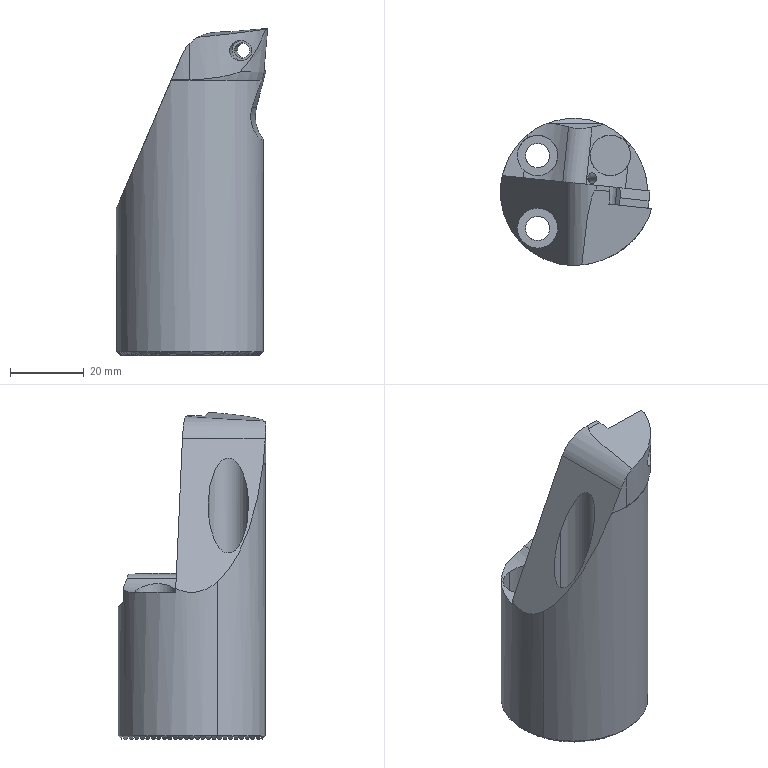NC program | Mastercam | posted with a generic post
Lines 22 to 750 of 11394:
(12 FEMR |TOOL - 1|DIA. OFF. - 1|LEN. - 1|TOOL DIA. - 12.)
N108 T1 M6
N110 G0 G55 G90 X47.529 Y29.275 C6. B-90. S3500 M3
N112 G43 H1 Z102.44
N114 Z4.44
N116 G1 Z2.69 F2000.
N118 X46.832 Y27.706 Z2.539 F2800.
N120 G3 X46.6 Y26.61 Z2.44 I2.468 J-1.096
N122 G1 Y26.
N124 X46.857 Y25.933
N126 G3 X49.366 Y25.751 I2.719 J20.13
N128 X56.385 Y25.697 I7.019 J457.418
N130 X58.173 Y25.7 J457.472
N132 G1 X58.58
N134 X73.217 Y25.712
N136 G3 X74.788 Y25.96 I-1.559 J14.923
N138 G2 X79.594 Y26.531 I10.889 J-71.178
N140 X85.304 Y27.044 I90.742 J-978.65
N142 G1 X85.71 Y27.079
N144 G2 X88.612 Y27.319 I14.877 J-162.688
N146 G1 X88.648
N148 G2 X91.848 Y26.431 J-6.209
N150 X94.413 Y23.878 I-3.935 J-6.52
N152 X95.771 Y20.319 I-9.343 J-5.604
N154 X96.172 Y16.703 I-22.913 J-4.367
N156 X96.263 Y11.23 I-164.754 J-5.473
N158 X96.26 Y10.372 I-164.845
N160 G1 X96.261 Y9.963
N162 X96.262 Y-20.063
N164 G2 X95.238 Y-23.24 I-6.113 J.217
N166 X92.516 Y-25.695 I-6.144 J4.075
N168 X89.126 Y-26.78 I-4.792 J9.131
N170 X86.426 Y-26.964 I-2.7 J19.725
N172 X85.595 Y-26.947 J19.909
N174 X80.026 Y-26.576 I4.415 J108.3
N176 X77.254 Y-26.296 I3.443 J47.898
N178 X75.239 Y-25.92 I6.779 J41.994
N180 G3 X72.669 Y-25.747 I-2.789 J-22.233
N182 X65.45 Y-25.696 I-7.219 J-514.472
N184 X63.445 Y-25.7 J-514.523
N186 G1 X63.038
N188 X46.6
N190 Y-26.514
N192 G3 X46.832 Y-27.609 Z2.514 I2.7
N194 G1 X47.529 Y-29.179 Z2.628
N196 G3 X47.993 Y-29.977 Z2.69 I3.871 J1.719
N198 X51.4 Y-31.696 I3.407 J2.517
N200 X51.486 Y-31.695 J4.236
N202 G1 X85.77 Y-31. F9500.
N204 G3 X97.868 Y-18.729 I-.251 J12.346
N206 G1 X98.099 Y19.214
N208 Y19.274
N210 G3 X88.634 Y29.049 I-9.78
N212 G1 X49.187 Y30.319
N214 G3 X49.132 Y30.32 I-.055 J-1.727
N216 X48.085 Y29.967 J-1.728
N218 X47.552 Y29.293 Z2.632 I1.047 J-1.375 F2800.
N220 G1 X47.529 Y29.241 Z2.628
N222 X46.832 Y27.672 Z2.514
N224 G3 X46.6 Y26.576 Z2.44 I2.468 J-1.096
N226 G1 Y25.966
N228 Y25.941
N230 G3 X47.322 Y25.742 I1.184 J2.896
N232 X50.202 Y25.481 I3.284 J20.205
N234 X56.326 Y25.4 I6.124 J231.975
N236 X57.331 Y25.403 J232.056
N238 G1 X57.737 Y25.402
N240 X71.868 Y25.405
N242 G3 X74.16 Y25.606 I-.455 J18.407
N244 G1 X74.56 Y25.656
N246 G2 X83.654 Y26.595 I27.944 J-226.233
N248 G1 X84.061 Y26.631
N250 G2 X86.741 Y26.858 I16.424 J-178.336
N252 X87.052 Y26.864 I.311 J-7.716
N254 X92.353 Y24.757 J-7.722
N256 X94.693 Y21.289 I-6.626 J-6.994
N258 X95.57 Y17.974 I-13.452 J-5.331
N260 X95.9 Y13.699 I-34.856 J-4.848
N262 X95.966 Y6.255 I-422.145 J-7.444
N264 X95.963 Y4.599 I-422.211
N266 G1 Y4.192
N268 X95.951 Y-18.459
N270 G2 X93.339 Y-23.853 I-7.737 J.417
N272 X89.684 Y-25.862 I-6.391 J7.299
N274 X86.31 Y-26.439 I-4.126 J13.967
N276 X84.545 Y-26.483 I-1.765 J35.346
N278 X82.028 Y-26.394 J35.39
N280 X77.974 Y-26.036 I2.926 J56.249
N282 G3 X74.974 Y-25.628 I-8.378 J-50.369
N284 X70.119 Y-25.427 I-4.903 J-59.734
N286 X62.633 Y-25.399 I-7.486 J-999.104
N288 X60.821 Y-25.4 J-999.132
N290 G1 X60.415
N292 X47.626 Y-25.411
N294 G3 X46.6 Y-25.508 I1.118 J-17.319
N296 G1 Y-25.915
N298 Y-26.322
N300 G3 X46.832 Y-27.418 Z2.514 I2.7
N302 G1 X47.529 Y-28.987 Z2.628
N304 G3 X47.967 Y-29.801 Z2.69 I5.542 J2.46
N306 X53.071 Y-32.591 I5.104 J3.274 F9500.
N308 X53.716 Y-32.556 J6.064
N310 G1 X86.509 Y-29.048
N312 G3 X97.568 Y-16.768 I-1.317 J12.305
N314 G1 X97.634 Y17.323
N316 Y17.345
N318 G3 X87.026 Y28.482 I-11.15
N320 G1 X49.293 Y30.322
N322 G3 X49.206 Y30.324 I-.087 J-1.793
N324 X48.066 Y29.915 J-1.795
N326 X47.566 Y29.257 Z2.634 I1.14 J-1.386 F2800.
N328 G1 X47.529 Y29.175 Z2.628
N330 X46.832 Y27.605 Z2.514
N332 G3 X46.6 Y26.51 Z2.44 I2.468 J-1.095
N334 G1 Y25.899
N336 Y25.867
N338 G3 X47.295 Y25.621 I1.309 J2.597
N340 X49.974 Y25.257 I3.398 J14.942
N342 X55.219 Y25.116 I5.245 J97.179
N344 X55.353 Y25.115 J97.32
N346 X60.423 Y25.101 I5.07 J930.161
N348 G1 X60.613
N350 X61.019
N352 X71.071 Y25.112
N354 G3 X74.684 Y25.394 I-1.302 J39.973
N356 X75.486 Y25.482 I-69.31 J635.193
N358 G2 X85.35 Y26.427 I36.383 J-327.653
N360 X85.873 Y26.443 I.523 J-8.656
N362 X92.552 Y23.301 J-8.672
N364 X94.646 Y19.395 I-8.696 J-7.175
N366 X95.414 Y15.35 I-18.846 J-5.675
N368 X95.636 Y10.046 I-67.384 J-5.48
N370 X95.664 Y2.602 I-985.697 J-7.444
N372 X95.663 Y1.031 I-985.725
N374 G1 Y.624
N376 X95.654 Y-16.85
N378 G2 X94.481 Y-21.108 I-8.896 J.161
N380 X91.007 Y-24.46 I-7.788 J4.595
N382 X87.055 Y-25.793 I-5.819 J10.73
N384 X83.54 Y-26.06 I-3.515 J23.029
N386 X82.887 Y-26.05 J23.296
N388 X77.474 Y-25.624 I.753 J44.179
N390 G3 X70.31 Y-25.146 I-7.489 J-58.236
N392 X60.515 Y-25.097 I-9.795 J-973.891
N394 X57.787 Y-25.1 J-973.94
N396 G1 X57.38
N398 X48.93 Y-25.107
N400 G3 X47.249 Y-25.217 I.087 J-14.256
N402 G2 X46.6 Y-25.332 I-4.342 J22.51
N404 G1 Y-25.739
N406 Y-26.146
N408 G3 X46.832 Y-27.242 Z2.514 I2.7
N410 G1 X47.529 Y-28.811 Z2.628
N412 G3 X47.967 Y-29.625 Z2.69 I5.563 J2.47
N414 X53.092 Y-32.428 I5.125 J3.284 F9500.
N416 X54.034 Y-32.355 J6.087
N418 G1 X86.769 Y-27.226
N420 G3 X97.268 Y-15.041 I-1.923 J12.272
N422 G1 X97.485 Y15.883
N424 Y15.968
N426 G3 X86.059 Y28.113 I-12.167
N428 G1 X49.574 Y30.338
N430 G3 X49.446 Y30.342 I-.128 J-2.094
N432 X48.075 Y29.832 J-2.098
N434 X47.529 Y29.095 Z2.628 I1.371 J-1.588 F2800.
N436 G1 X46.832 Y27.526 Z2.514
N438 G3 X46.6 Y26.43 Z2.44 I2.468 J-1.096
N440 G1 Y25.82
N442 Y25.783
N444 G3 X47.27 Y25.501 I1.407 J2.405
N446 X49.799 Y25.047 I3.498 J12.216
N448 X54.651 Y24.836 I5.066 J60.597
N450 X63.195 Y24.799 I8.544 J976.208
N452 X65.158 Y24.8 J976.245
N454 G1 X65.565
N456 G3 X66.808 Y24.797 I1.243 J274.393
N458 X70.699 Y24.825 J274.396
N460 X75.601 Y25.204 I-2.579 J65.269
N462 G1 X76.004 Y25.245
N464 G2 X83.915 Y26. I42.144 J-400.038
N466 X84.724 Y26.031 I.809 J-10.529
N468 X87.755 Y25.586 J-10.56
N470 X92.529 Y22.101 I-2.915 J-9.004
N472 X94.427 Y18.073 I-10.224 J-7.28
N474 X95.128 Y13.927 I-21.982 J-5.849
N476 X95.339 Y8.254 I-78.186 J-5.743
N478 X95.364 Y1.244 I-984.987 J-7.01
N480 X95.363 Y.062 I-985.012
N482 G1 Y-.345
N484 X95.352 Y-15.565
N486 G2 X94.587 Y-19.353 I-10.488 J.146
N488 X90.687 Y-23.783 I-8.729 J3.753
N490 X86.513 Y-25.312 I-6.351 J10.875
N492 X82.616 Y-25.647 I-3.897 J22.504
N494 X81.802 Y-25.633 J22.839
N496 X77.357 Y-25.289 I2.204 J57.489
N498 G3 X68.875 Y-24.837 I-8.75 J-84.258
N500 X60.513 Y-24.799 I-8.362 J-930.633
N502 X58.769 Y-24.801 J-930.671
N504 G1 X58.362
N506 X49.898 Y-24.808
N508 X49.838
N510 G3 X47.426 Y-24.976 J-17.429
N512 X46.6 Y-25.163 I1.255 J-7.445
N514 G1 Y-25.57
N516 Y-25.977
N518 G3 X46.832 Y-27.073 Z2.514 I2.7
N520 G1 X47.529 Y-28.642 Z2.628
N522 G3 X47.967 Y-29.456 Z2.69 I5.556 J2.466
N524 X53.085 Y-32.255 I5.118 J3.28 F9500.
N526 X54.152 Y-32.161 J6.079
N528 G1 X86.738 Y-26.352
N530 G3 X96.968 Y-14.185 I-2.177 J12.214
N532 G1 X97.079 Y15.053
N534 Y15.101
N536 G3 X85.297 Y27.742 I-12.672
N538 G1 X49.462 Y30.265
N540 G3 X49.328 Y30.27 I-.134 J-1.901
N542 X48.041 Y29.769 J-1.906
N544 X47.586 Y29.137 Z2.638 I1.287 J-1.405 F2800.
N546 G1 X47.529 Y29.008 Z2.628
N548 X46.832 Y27.439 Z2.514
N550 G3 X46.6 Y26.343 Z2.44 I2.468 J-1.096
N552 G1 Y25.733
N554 Y25.692
N556 G3 X47.246 Y25.381 I1.486 J2.256
N558 X49.656 Y24.848 I3.594 J10.545
N560 X53.998 Y24.57 I5.035 J44.572
N562 X62.635 Y24.498 I8.637 J517.551
N564 X64.445 Y24.501 J517.623
N566 G1 X64.852
N568 G3 X66.254 Y24.496 I1.402 J207.057
N570 X70.379 Y24.537 J207.062
N572 X76.13 Y24.965 I-3.438 J85.072
N574 X76.935 Y25.044 I-88.258 J904.631
N576 G1 X77.34 Y25.084
N578 G2 X82.786 Y25.591 I34.321 J-339.181
N580 X83.761 Y25.629 I.975 J-12.402
N582 X86.229 Y25.382 J-12.44
N584 X91.998 Y21.636 I-2.123 J-9.585
N586 X93.961 Y17.697 I-10.303 J-7.593
N588 X94.761 Y13.523 I-20.947 J-6.177
N590 X95.021 Y8.208 I-64.782 J-5.834
N592 X95.067 Y-1.223 I-975.08 J-9.431
N594 X95.063 Y-3.68 I-975.126
N596 G1 Y-4.087
N598 X95.049 Y-14.413
N600 G2 X94.522 Y-17.822 I-12.377 J.17
N602 X90.27 Y-23.216 I-9.382 J3.023
N604 X86.176 Y-24.816 I-6.647 J10.966
N606 X82.02 Y-25.229 I-4.156 J20.707
N608 X81.378 Y-25.22 J21.12
N610 X76.991 Y-24.938 I2.34 J70.796
N612 G3 X67.609 Y-24.531 I-9.629 J-113.557
N614 X60.091 Y-24.501 I-7.518 J-940.281
N616 G1 X59.115
N618 X58.709
N620 G3 X56.458 Y-24.498 I-2.251 J-986.24
N622 X50.281 Y-24.518 J-986.243
N624 X47.503 Y-24.755 I.088 J-17.442
N626 X46.6 Y-24.999 I1.506 J-7.359
N628 G1 Y-25.406
N630 Y-25.813
N632 G3 X46.832 Y-26.909 Z2.514 I2.7
N634 G1 X47.529 Y-28.478 Z2.628
N636 G3 X47.968 Y-29.291 Z2.69 I5.494 J2.439
N638 X53.023 Y-32.05 I5.055 J3.252 F9500.
N640 X53.949 Y-31.978 J6.011
N642 G1 X86.277 Y-26.939
N644 G3 X96.654 Y-14.952 I-1.889 J12.121
N646 G1 X96.965 Y13.493
N648 G3 X96.966 Y13.644 I-13.78 J.151
N650 X84.307 Y27.379 I-13.781
N652 G1 X49.534 Y30.219
N654 G3 X49.376 Y30.225 I-.158 J-1.939
N656 X48.029 Y29.685 J-1.945
N658 X47.597 Y29.069 Z2.639 I1.347 J-1.405 F2800.
N660 G1 X47.529 Y28.916 Z2.628
N662 X46.832 Y27.346 Z2.514
N664 G3 X46.6 Y26.251 Z2.44 I2.468 J-1.095
N666 G1 Y25.64
N668 Y25.597
N670 G3 X47.223 Y25.261 I1.504 J2.039
N672 X49.535 Y24.658 I3.688 J9.408
N674 X53.768 Y24.306 I5.138 J36.114
N676 X61.495 Y24.203 I7.727 J289.202
N678 X62.537 Y24.204 J289.305
N680 G1 X62.942
N682 G3 X64.779 Y24.199 I1.837 J320.857
N684 X69.712 Y24.236 J320.862
N686 X76.27 Y24.686 I-3.143 J93.901
N688 X78.285 Y24.878 I-90.027 J956.941
N690 G1 X78.691 Y24.916
N692 G2 X82.181 Y25.215 I10.21 J-98.931
N694 X82.967 Y25.239 I.786 J-12.621
N696 X85.914 Y24.891 J-12.645
N698 X91.707 Y20.905 I-2.563 J-9.928
N700 X93.505 Y17.335 I-10.653 J-7.603
N702 X94.392 Y13.145 I-20.202 J-6.468
N704 X94.706 Y7.779 I-57.675 J-6.064
N706 X94.767 Y-1.755 I-745.007 J-9.534
N708 X94.763 Y-4.132 I-745.068
N710 G1 Y-4.539
N712 X94.751 Y-13.204
N714 G2 X94.415 Y-16.251 I-14.842 J.094
N716 X89.662 Y-22.806 I-9.994 J2.246
N718 X85.632 Y-24.38 I-6.749 J11.333
N720 X81.446 Y-24.81 I-4.186 J20.176
N722 X81.331 Y-24.809 J20.606
N724 X76.899 Y-24.613 I.618 J63.945
N726 G3 X65.922 Y-24.222 I-10.977 J-153.939
N728 G1 X65.828
N730 G3 X60.162 Y-24.203 I-6.074 J-976.985
N732 G1 X59.756
N734 G3 X57.131 Y-24.199 I-2.625 J-837.057
N736 X50.926 Y-24.222 J-837.061
N738 X48.057 Y-24.442 I.176 J-21.093
N740 X46.6 Y-24.837 I.987 J-6.516
N742 G1 Y-25.244
N744 Y-25.651
N746 G3 X46.832 Y-26.747 Z2.514 I2.7
N748 G1 X47.529 Y-28.316 Z2.628
N750 G3 X47.968 Y-29.129 Z2.69 I5.461 J2.424
N752 X52.99 Y-31.867 I5.022 J3.237 F9500.
N754 X53.937 Y-31.792 J5.975
N756 G1 X86.05 Y-26.64
N758 G3 X96.31 Y-14.865 I-1.931 J12.04
N760 G1 X96.892 Y11.859
N762 G3 X96.895 Y12.18 I-14.731 J.321
N764 X83.594 Y26.844 I-14.734
N766 G1 X49.602 Y30.167
N768 G3 X49.41 Y30.176 I-.192 J-1.958
N770 X48.017 Y29.597 J-1.967
N772 X47.612 Y29.007 Z2.642 I1.393 J-1.388 F2800.
N774 G1 X47.529 Y28.819 Z2.628
N776 X46.832 Y27.25 Z2.514
N778 G3 X46.6 Y26.154 Z2.44 I2.468 J-1.096
N780 G1 Y25.544
N782 Y25.499
N784 G3 X47.202 Y25.14 I1.558 J1.932
N786 X49.431 Y24.474 I3.779 J8.58
N788 X53.564 Y24.048 I5.24 J30.585
N790 X60.61 Y23.911 I7.046 J180.595
N792 G1 X61.061
N794 G3 X63.085 Y23.905 I3.774 J972.824
N796 G1 X63.491
N798 G3 X65.052 Y23.898 I1.561 J184.658
N800 X70.204 Y23.97 J184.665
N802 X77.226 Y24.481 I-5.685 J126.675
N804 X78.032 Y24.556 I-83.251 J898.938
N806 G1 X78.437 Y24.594
N808 G2 X81.574 Y24.838 I6.786 J-66.905
N810 X82.215 Y24.853 I.641 J-13.291
N812 X85.185 Y24.517 J-13.306
N814 X91.413 Y20.216 I-2.521 J-10.31
N816 X93.241 Y16.434 I-11.335 J-7.813
N818 X94.135 Y11.832 I-22.073 J-6.673
N820 X94.416 Y6.113 I-68.472 J-6.238
N822 X94.466 Y-3.799 I-988.079 J-9.912
N824 X94.463 Y-6.183 I-988.129
N826 G1 Y-6.591
N828 G2 X94.466 Y-8.052 I-424.572 J-1.461
N830 X94.443 Y-12.442 I-424.575
N832 X94.043 Y-15.737 I-15.177 J.172
N834 X89.131 Y-22.378 I-10.309 J2.487
N836 X84.862 Y-24.004 I-6.872 J11.631
N838 X80.688 Y-24.405 I-4.174 J21.504
N840 G1 X80.641
N842 G2 X75.848 Y-24.232 I.425 J78.093
N844 G3 X64.583 Y-23.917 I-11.265 J-201.327
N846 G1 X64.307
N848 G3 X60.663 Y-23.905 I-5.051 J-995.672
N850 G1 X60.257 Y-23.904
N852 G3 X57.518 Y-23.898 I-2.739 J-654.676
N854 X51.439 Y-23.927 J-654.682
N856 X48.205 Y-24.195 I.142 J-21.353
N858 X46.6 Y-24.677 I1.11 J-6.602
N860 G1 Y-25.084
N862 Y-25.491
N864 G3 X46.832 Y-26.587 Z2.514 I2.7
N866 G1 X47.529 Y-28.156 Z2.628
N868 G3 X47.968 Y-28.969 Z2.69 I5.497 J2.44
N870 X53.026 Y-31.73 I5.058 J3.253 F9500.
N872 X54.264 Y-31.601 J6.014
N874 G1 X86.304 Y-24.856
N876 G3 X96.048 Y-12.988 I-2.529 J12.01
N878 G1 X96.331 Y11.67
N880 G3 X96.332 Y11.841 I-14.88 J.171
N882 X82.991 Y26.643 I-14.881
N884 G1 X49.669 Y30.111
N886 G3 X49.461 Y30.122 I-.208 J-2.003
N888 X48.009 Y29.503 J-2.014
N890 X47.62 Y28.925 Z2.643 I1.452 J-1.395 F2800.
N892 G1 X47.529 Y28.719 Z2.628
N894 X46.832 Y27.15 Z2.514
N896 G3 X46.6 Y26.054 Z2.44 I2.468 J-1.096
N898 G1 Y25.444
N900 Y25.397
N902 G3 X47.182 Y25.019 I1.601 J1.83
N904 X49.339 Y24.294 I3.864 J7.931
N906 X53.012 Y23.821 I5.101 J25.076
N908 X59.612 Y23.626 I6.695 J114.795
N910 X63.521 Y23.606 I3.909 J377.91
N912 X68.801 Y23.642 J377.93
N914 X76.991 Y24.164 I-3.418 J118.146
N916 G1 X77.393 Y24.2
N918 G2 X80.964 Y24.463 I6.548 J-64.625
N920 X81.518 Y24.474 I.554 J-13.576
N922 X84.842 Y24.062 J-13.587
N924 X90.937 Y19.818 I-2.819 J-10.548
N926 X92.986 Y15.537 I-11.573 J-8.172
N928 X93.83 Y10.997 I-23.493 J-6.715
N930 X94.112 Y5.291 I-70.353 J-6.336
N932 X94.166 Y-4.875 I-951.681 J-10.166
N934 X94.163 Y-7.416 I-951.735
N936 G1 Y-7.824
N938 G2 X94.167 Y-8.784 I-111.645 J-.96
N940 X94.116 Y-12.154 I-111.649
N942 X93.496 Y-15.858 I-14.33 J.496
N944 X88.343 Y-22.12 I-10.435 J3.336
N946 X83.863 Y-23.678 I-6.827 J12.417
N948 X79.729 Y-24.021 I-4.134 J24.752
N950 X79.296 Y-24.017 J25.095
N952 X74.214 Y-23.843 I2.351 J143.346
N954 G3 X62.806 Y-23.61 I-11.408 J-279.326
N956 X62.213 Y-23.611 J-279.559
N958 G1 X61.808 Y-23.61
N960 G3 X58.24 Y-23.601 I-3.568 J-722.458
N962 X52.171 Y-23.626 J-722.467
N964 X48.805 Y-23.868 I.187 J-26.164
N966 X47.012 Y-24.333 I1.095 J-7.901
N968 G1 X46.6 Y-24.519
N970 Y-25.333
N972 G3 X46.832 Y-26.428 Z2.514 I2.7
N974 G1 X47.529 Y-27.998 Z2.628
N976 G3 X47.968 Y-28.811 Z2.69 I5.47 J2.429
N978 X52.999 Y-31.554 I5.031 J3.242 F9500.
N980 X54.274 Y-31.417 J5.985
N982 G1 X86.11 Y-24.477
N984 G3 X95.722 Y-12.734 I-2.601 J11.935
N986 G1 X96.091 Y10.798
N988 G3 X96.093 Y11.035 I-15.119 J.237
N990 X82.79 Y26.046 I-15.121
N992 G1 X49.732 Y30.049
N994 G3 X49.488 Y30.064 I-.244 J-2.011
N996 X47.997 Y29.408 J-2.026
N998 X47.637 Y28.86 Z2.646 I1.491 J-1.37 F2800.
N1000 G1 X47.529 Y28.617 Z2.628
N1002 X46.832 Y27.047 Z2.514
N1004 G3 X46.6 Y25.952 Z2.44 I2.468 J-1.095
N1006 G1 Y25.341
N1008 Y25.292
N1010 G3 X47.162 Y24.898 I1.643 J1.743
N1012 X49.543 Y24.051 I4.181 J7.987
N1014 X53.577 Y23.525 I5.516 J26.579
N1016 X60.588 Y23.325 I7.121 J126.428
N1018 X63.663 Y23.306 I3.075 J245.327
N1020 X69.333 Y23.371 J245.346
N1022 X77.586 Y23.92 I-5.319 J142.271
N1024 G2 X80.901 Y24.096 I3.759 J-39.482
N1026 G1 X80.972
N1028 G2 X85.192 Y23.392 J-12.996
N1030 X90.675 Y19.145 I-3.826 J-10.602
N1032 X92.572 Y15.195 I-11.875 J-8.133
N1034 X93.48 Y10.642 I-22.87 J-6.928
N1036 X93.801 Y4.903 I-64.996 J-6.506
N1038 X93.867 Y-5.157 I-771.637 J-10.06
N1040 X93.863 Y-7.415 I-771.703
N1042 X93.866 Y-8.121 I-98.401 J-.706
N1044 X93.813 Y-11.334 I-98.404
N1046 X93.271 Y-14.9 I-15.59 J.543
N1048 X87.895 Y-21.681 I-10.785 J3.03
N1050 X83.748 Y-23.192 I-6.877 J12.426
N1052 X79.154 Y-23.638 I-4.636 J23.902
N1054 G1 X78.899
N1056 G2 X74.012 Y-23.528 J109.207
N1058 G3 X61.356 Y-23.306 I-12.656 J-360.414
N1060 X60.35 Y-23.308 J-360.636
N1062 G1 X59.945 Y-23.307
N1064 G3 X57.71 Y-23.3 I-2.235 J-377.946
N1066 X52.366 Y-23.338 J-377.953
N1068 X49.01 Y-23.603 I.358 J-25.905
N1070 X46.993 Y-24.165 I1.147 J-8.015
N1072 G1 X46.6 Y-24.361
N1074 Y-25.175
N1076 G3 X46.832 Y-26.27 Z2.514 I2.7
N1078 G1 X47.529 Y-27.84 Z2.628
N1080 G3 X47.968 Y-28.652 Z2.69 I5.448 J2.419
N1082 X52.977 Y-31.382 I5.009 J3.231 F9500.
N1084 X54.303 Y-31.232 J5.961
N1086 G1 X85.935 Y-24.013
N1088 G3 X95.389 Y-12.455 I-2.707 J11.86
N1090 G1 X95.93 Y9.33
N1092 G3 X95.935 Y9.732 I-16.2 J.402
N1094 X81.829 Y25.801 I-16.205
N1096 G1 X49.794 Y29.984
N1098 G3 X49.528 Y30.001 I-.266 J-2.039
N1100 X47.988 Y29.309 J-2.056
N1102 X47.648 Y28.779 Z2.648 I1.54 J-1.364 F2800.
N1104 G1 X47.529 Y28.512 Z2.628
N1106 X46.832 Y26.942 Z2.514
N1108 G3 X46.6 Y25.847 Z2.44 I2.468 J-1.095
N1110 G1 Y25.236
N1112 Y25.185
N1114 G3 X47.143 Y24.775 I1.675 J1.655
N1116 X49.457 Y23.873 I4.249 J7.479
N1118 X53.414 Y23.281 I5.61 J23.96
N1120 X59.97 Y23.039 I6.93 J98.96
N1122 X63.541 Y23.01 I3.571 J222.166
N1124 X69.491 Y23.09 J222.195
N1126 X76.977 Y23.57 I-5.806 J149.136
N1128 G2 X80.283 Y23.727 I3.551 J-39.856
N1130 G1 X80.299
N1132 G2 X84.454 Y23.08 J-13.648
N1134 X90.406 Y18.502 I-3.674 J-10.935
N1136 X92.327 Y14.331 I-12.519 J-8.296
N1138 X93.183 Y9.833 I-24.284 J-6.948
N1140 X93.498 Y4.112 I-67.468 J-6.582
N1142 X93.562 Y-4.885 I-635.778 J-8.997
N1144 X93.544 Y-9.54 I-635.842
N1146 X93.255 Y-12.954 I-22.926 J.221
N1148 X91.05 Y-18.141 I-11.77 J1.941
N1150 X86.305 Y-21.824 I-9.379 J7.186
N1152 X81.787 Y-23.04 I-6.47 J15.044
N1154 X77.661 Y-23.285 I-4.126 J34.615
N1156 X77.018 Y-23.279 J34.86
N1158 X70.421 Y-23.119 I5.809 J376.107
N1160 G3 X58.85 Y-23.007 I-11.571 J-595.59
N1162 X53.165 Y-23.034 J-595.702
N1164 X49.382 Y-23.309 I.31 J-30.413
N1166 X47.177 Y-23.901 I1.264 J-9.117
N1168 X46.6 Y-24.203 I2.367 J-5.22
N1170 G1 Y-24.61
N1172 Y-25.017
N1174 G3 X46.832 Y-26.112 Z2.514 I2.7
N1176 G1 X47.529 Y-27.682 Z2.628
N1178 G3 X47.969 Y-28.494 Z2.69 I5.376 J2.387
N1180 X52.905 Y-31.177 I4.936 J3.199 F9500.
N1182 X54.133 Y-31.048 J5.882
N1184 G1 X85.44 Y-24.368
N1186 G3 X94.923 Y-13.266 I-2.504 J11.74
N1188 G1 X95.997 Y6.912
N1190 G3 X96.022 Y7.858 I-17.767 J.946
N1192 X80.726 Y25.474 I-17.792
N1194 G1 X49.394 Y29.915
N1196 G3 X49.183 Y29.93 I-.211 J-1.488
N1198 X47.92 Y29.241 J-1.503
N1200 X47.81 Y29.037 Z2.674 I1.263 J-.814 F2800.
N1202 G1 X47.529 Y28.404 Z2.628
N1204 X46.832 Y26.835 Z2.514
N1206 G3 X46.6 Y25.739 Z2.44 I2.468 J-1.096
N1208 G1 Y25.129
N1210 Y25.076
N1212 G3 X47.124 Y24.653 I1.701 J1.572
N1214 X49.376 Y23.699 I4.311 J7.041
N1216 X53.261 Y23.042 I5.717 J21.98
N1218 X59.364 Y22.759 I6.886 J82.709
N1220 X63.507 Y22.717 I4.143 J204.432
N1222 X69.659 Y22.81 J204.474
N1224 X76.799 Y23.255 I-7.288 J174.458
N1226 G2 X79.388 Y23.36 I2.589 J-31.88
N1228 X80.221 Y23.349 J-31.985
N1230 X84.403 Y22.537 I-.426 J-13.379
N1232 X89.953 Y18.147 I-4.205 J-11.018
N1234 X92.004 Y13.749 I-12.567 J-8.538
N1236 X92.911 Y8.801 I-25.955 J-7.313
N1238 X93.208 Y2.699 I-78.781 J-6.892
N1240 X93.258 Y-4.452 I-515.283 J-7.151
N1242 X93.238 Y-8.917 I-515.333
N1244 X92.892 Y-12.597 I-23.018 J.308
N1246 X90.42 Y-17.995 I-11.873 J2.172
N1248 X85.673 Y-21.491 I-9.385 J7.773
N1250 X81.227 Y-22.664 I-6.518 J15.692
N1252 X76.84 Y-22.932 I-4.387 J35.828
N1254 X76.485 Y-22.93 J36.096
N1256 X69.864 Y-22.809 I2.952 J343.122
N1258 G3 X59.075 Y-22.711 I-10.789 J-592.181
N1260 X53.802 Y-22.734 J-592.279
N1262 X49.942 Y-22.986 I.361 J-35.165
N1264 X47.574 Y-23.551 I1.332 J-10.834
N1266 X46.91 Y-23.862 I1.381 J-3.812
N1268 X46.6 Y-24.135 I.626 J-1.024
N1270 G1 Y-24.542
N1272 G3 X46.832 Y-25.637 Z2.514 I2.7
N1274 G1 X47.529 Y-27.207 Z2.628
N1276 G3 X47.969 Y-28.019 Z2.69 I5.401 J2.398
N1278 X52.93 Y-30.718 I4.961 J3.21 F9500.
N1280 X54.343 Y-30.547 J5.909
N1282 G1 X85.569 Y-22.859
N1284 G3 X94.741 Y-11.488 I-2.884 J11.711
N1286 G1 X95.292 Y8.054
N1288 G3 X95.299 Y8.529 I-16.794 J.475
N1290 X81.01 Y25.141 I-16.801
N1292 G1 X49.91 Y29.843
N1294 G3 X49.595 Y29.867 I-.315 J-2.082
N1296 X47.972 Y29.102 J-2.106
N1298 X47.671 Y28.615 Z2.652 I1.623 J-1.341 F2800.
N1300 G1 X47.529 Y28.295 Z2.628
N1302 X46.832 Y26.725 Z2.514
N1304 G3 X46.6 Y25.63 Z2.44 I2.468 J-1.095
N1306 G1 Y25.019
N1308 Y24.965
N1310 G3 X47.106 Y24.529 I1.713 J1.481
N1312 X49.299 Y23.527 I4.367 J6.655
N1314 X52.764 Y22.847 I5.556 J19.137
N1316 X58.379 Y22.496 I6.713 J62.22
N1318 X63.52 Y22.425 I5.141 J186.369
N1320 X70.225 Y22.545 J186.44
N1322 X76.638 Y22.937 I-9.493 J208.339
N1324 G2 X78.563 Y23.005 I1.925 J-27.328
N1326 X80.164 Y22.958 J-27.396
N1328 X85.33 Y21.521 I-.803 J-12.89
N1330 X90.053 Y16.96 I-5.857 J-10.792
N1332 X91.902 Y12.377 I-14.336 J-8.451
N1334 X92.658 Y7.548 I-29.953 J-7.158
N1336 X92.919 Y1.087 I-93.665 J-7.03
N1338 X92.954 Y-4.315 I-415.985 J-5.402
N1340 X92.938 Y-8.054 I-416.02
N1342 X92.646 Y-11.624 I-25.907 J.322
N1344 X90.696 Y-16.663 I-12.573 J1.967
N1346 X85.655 Y-20.897 I-10.005 J6.795
N1348 X80.945 Y-22.257 I-7.013 J15.452
N1350 X76.189 Y-22.583 I-4.783 J34.883
N1352 G1 X76.165
N1354 G2 X69.529 Y-22.503 J273.119
N1356 G3 X59.435 Y-22.415 I-10.094 J-576.019
N1358 X54.267 Y-22.437 J-576.107
N1360 X50.361 Y-22.684 I.44 J-38.026
N1362 X47.68 Y-23.314 I1.278 J-11.45
N1364 X46.808 Y-23.789 I1.386 J-3.59
N1366 G1 X46.6 Y-23.918
N1368 Y-24.731
N1370 G3 X46.832 Y-25.827 Z2.514 I2.7
N1372 G1 X47.529 Y-27.396 Z2.628
N1374 G3 X47.969 Y-28.209 Z2.69 I5.402 J2.398
N1376 X52.931 Y-30.908 I4.962 J3.211 F9500.
N1378 X54.474 Y-30.703 J5.91
N1380 G1 X85.505 Y-22.308
N1382 G3 X94.408 Y-11.112 I-3.151 J11.643
N1384 G1 X95.076 Y6.902
N1386 G3 X95.088 Y7.562 I-17.792 J.66
N1388 X80.087 Y25.144 I-17.804
N1390 G1 X50.591 Y29.846
N1392 G3 X50.141 Y29.882 I-.45 J-2.822
N1394 X48.033 Y28.954 J-2.858
N1396 X47.529 Y28.183 Z2.628 I2.108 J-1.93 F2800.
N1398 G1 X46.832 Y26.614 Z2.514
N1400 G3 X46.6 Y25.518 Z2.44 I2.468 J-1.096
N1402 G1 Y24.908
N1404 Y24.851
N1406 G3 X47.088 Y24.406 I1.703 J1.375
N1408 X49.225 Y23.358 I4.417 J6.309
N1410 X52.63 Y22.622 I5.641 J17.836
N1412 X58.192 Y22.22 I6.832 J55.853
N1414 X63.605 Y22.132 I5.413 J166.815
N1416 X71.583 Y22.322 J166.903
N1418 X76.045 Y22.593 I-15.443 J292.002
N1420 G2 X77.899 Y22.652 I1.854 J-28.928
N1422 X79.527 Y22.606 J-28.987
N1424 X83.948 Y21.583 I-.809 J-13.557
N1426 X89.446 Y16.898 I-4.907 J-11.326
N1428 X91.376 Y12.585 I-13.578 J-8.666
N1430 X92.279 Y7.681 I-26.875 J-7.48
N1432 X92.597 Y1.574 I-77.159 J-7.083
N1434 X92.65 Y-3.979 I-293.347 J-5.553
N1436 X92.627 Y-7.628 I-293.4
N1438 X92.301 Y-11.221 I-25.036 J.459
N1440 X90.334 Y-16.206 I-12.743 J2.147
N1442 X85.364 Y-20.431 I-10.152 J6.908
N1444 X80.945 Y-21.806 I-7.136 J15.135
N1446 X76.133 Y-22.232 I-5.281 J32.263
N1448 X73.697 Y-22.25 I-2.436 J168.148
N1450 X69.821 Y-22.205 J168.166
N1452 G1 X69.415 Y-22.199
N1454 G3 X59.629 Y-22.117 I-9.786 J-586.993
N1456 X54.942 Y-22.136 J-587.075
N1458 X50.644 Y-22.398 I.299 J-40.313
N1460 X47.924 Y-23.025 I1.35 J-12.069
N1462 X46.6 Y-23.75 I1.995 J-5.216
N1464 G1 Y-24.157
N1466 Y-24.564
N1468 G3 X46.832 Y-25.66 Z2.514 I2.7
N1470 G1 X47.529 Y-27.229 Z2.628
N1472 G3 X47.969 Y-28.041 Z2.69 I5.343 J2.372
N1474 X52.872 Y-30.703 I4.903 J3.184 F9500.
N1476 X54.371 Y-30.507 J5.846
N1478 G1 X85.093 Y-22.356
N1480 G3 X93.922 Y-11.819 I-3.06 J11.532
N1482 G1 X95.182 Y3.234
N1484 G3 X95.253 Y4.937 I-20.345 J1.703
N1486 X78.256 Y25.065 I-20.416
N1488 G1 X50.663 Y29.751
N1490 G3 X50.178 Y29.792 I-.485 J-2.857
N1492 X48.032 Y28.842 J-2.898
N1494 X47.529 Y28.07 Z2.628 I2.146 J-1.948 F2800.
N1496 G1 X46.832 Y26.501 Z2.514
N1498 G3 X46.6 Y25.405 Z2.44 I2.468 J-1.096
N1500 G1 Y24.795
N1502 Y24.736
N1504 G3 X47.225 Y24.164 I1.962 J1.517
N1506 X49.419 Y23.1 I4.616 J6.722
N1508 X53.19 Y22.305 I6.048 J19.357
N1510 X58.787 Y21.919 I6.952 J60.069
N1512 X63.829 Y21.84 I5.042 J160.832
N1514 X75.021 Y22.23 J160.911
N1516 G2 X77.205 Y22.304 I2.184 J-32.35
N1518 X78.893 Y22.26 J-32.424
N1520 X83.557 Y21.183 I-.784 J-14.032
N1522 X89.02 Y16.554 I-5.009 J-11.451
N1524 X90.992 Y12.266 I-13.55 J-8.83
N1526 X91.941 Y7.352 I-26.336 J-7.633
N1528 X92.287 Y1.224 I-73.216 J-7.208
N1530 X92.343 Y-3.669 I-214.165 J-4.893
N1532 X92.314 Y-7.202 I-214.221
N1534 X91.958 Y-10.813 I-24.465 J.589
N1536 X89.777 Y-16.04 I-12.784 J2.265
N1538 X84.793 Y-20.106 I-10.18 J7.392
N1540 X80.173 Y-21.491 I-7.303 J15.959
N1542 X75.418 Y-21.899 I-5.363 J34.663
N1544 X72.399 Y-21.923 I-3.019 J190.485
N1546 X68.705 Y-21.887 J190.509
N1548 G1 X68.298 Y-21.882
N1550 G3 X59.991 Y-21.821 I-8.307 J-564.3
N1552 X55.435 Y-21.839 J-564.361
N1554 X51.092 Y-22.09 I.351 J-43.723
N1556 X48.256 Y-22.702 I1.401 J-13.372
N1558 X46.6 Y-23.587 I1.768 J-5.299
N1560 G1 Y-23.994
N1562 Y-24.401